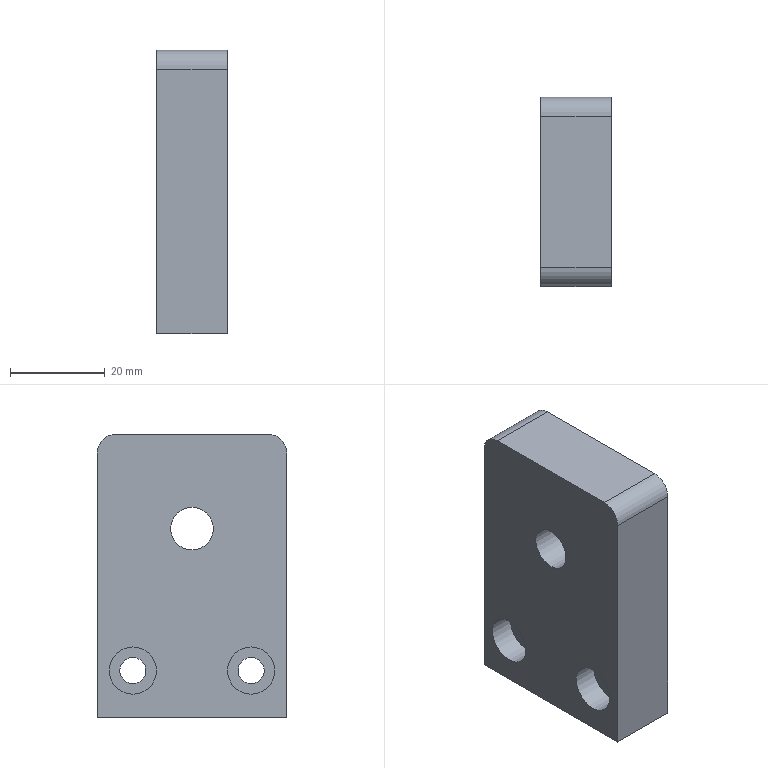Part | NX | 1 solid | 17 faces | box 15 x 40 x 60 mm | volume 32666 mm3 | plane 9 | cylinder 8 | commonest cylinder face diameters 5.5 x2 8 x2 10 x2 9 x1 15 x1
STEP:
#1=CARTESIAN_POINT('',(0.,-20.,-30.));
#2=VERTEX_POINT('',#1);
#3=CARTESIAN_POINT('',(0.,20.,-30.));
#4=VERTEX_POINT('',#3);
#5=CARTESIAN_POINT('',(0.,20.,-30.));
#6=DIRECTION('',(0.,1.,0.));
#7=VECTOR('',#6,1000.);
#8=LINE('',#5,#7);
#9=EDGE_CURVE('',#2,#4,#8,.T.);
#10=ORIENTED_EDGE('',*,*,#9,.T.);
#11=CARTESIAN_POINT('',(15.,20.,-30.));
#12=VERTEX_POINT('',#11);
#13=CARTESIAN_POINT('',(15.,20.,-30.));
#14=DIRECTION('',(-1.,0.,0.));
#15=VECTOR('',#14,1000.);
#16=LINE('',#13,#15);
#17=EDGE_CURVE('',#12,#4,#16,.T.);
#18=ORIENTED_EDGE('',*,*,#17,.F.);
#19=CARTESIAN_POINT('',(15.,-20.,-30.));
#20=VERTEX_POINT('',#19);
#21=CARTESIAN_POINT('',(15.,20.,-30.));
#22=DIRECTION('',(0.,1.,0.));
#23=VECTOR('',#22,1000.);
#24=LINE('',#21,#23);
#25=EDGE_CURVE('',#20,#12,#24,.T.);
#26=ORIENTED_EDGE('',*,*,#25,.F.);
#27=CARTESIAN_POINT('',(15.,-20.,-30.));
#28=DIRECTION('',(-1.,0.,0.));
#29=VECTOR('',#28,1000.);
#30=LINE('',#27,#29);
#31=EDGE_CURVE('',#20,#2,#30,.T.);
#32=ORIENTED_EDGE('',*,*,#31,.T.);
#33=EDGE_LOOP('',(#10,#18,#26,#32));
#34=FACE_BOUND('',#33,.T.);
#35=CARTESIAN_POINT('',(15.,20.,-30.));
#36=DIRECTION('',(0.,0.,1.));
#37=DIRECTION('',(1.,0.,0.));
#38=AXIS2_PLACEMENT_3D('',#35,#36,#37);
#39=PLANE('',#38);
#40=ADVANCED_FACE('',(#34),#39,.F.);
#41=CARTESIAN_POINT('',(0.,20.,26.));
#42=VERTEX_POINT('',#41);
#43=CARTESIAN_POINT('',(0.,20.,30.));
#44=DIRECTION('',(0.,0.,1.));
#45=VECTOR('',#44,1000.);
#46=LINE('',#43,#45);
#47=EDGE_CURVE('',#4,#42,#46,.T.);
#48=ORIENTED_EDGE('',*,*,#47,.T.);
#49=CARTESIAN_POINT('',(15.,20.,26.));
#50=VERTEX_POINT('',#49);
#51=CARTESIAN_POINT('',(15.,20.,26.));
#52=DIRECTION('',(-1.,0.,0.));
#53=VECTOR('',#52,1000.);
#54=LINE('',#51,#53);
#55=EDGE_CURVE('',#42,#50,#54,.F.);
#56=ORIENTED_EDGE('',*,*,#55,.T.);
#57=CARTESIAN_POINT('',(15.,20.,30.));
#58=DIRECTION('',(0.,0.,1.));
#59=VECTOR('',#58,1000.);
#60=LINE('',#57,#59);
#61=EDGE_CURVE('',#12,#50,#60,.T.);
#62=ORIENTED_EDGE('',*,*,#61,.F.);
#63=ORIENTED_EDGE('',*,*,#17,.T.);
#64=EDGE_LOOP('',(#48,#56,#62,#63));
#65=FACE_BOUND('',#64,.T.);
#66=CARTESIAN_POINT('',(15.,20.,30.));
#67=DIRECTION('',(0.,-1.,0.));
#68=DIRECTION('',(0.,0.,-1.));
#69=AXIS2_PLACEMENT_3D('',#66,#67,#68);
#70=PLANE('',#69);
#71=ADVANCED_FACE('',(#65),#70,.F.);
#72=CARTESIAN_POINT('',(0.,16.,30.));
#73=VERTEX_POINT('',#72);
#74=CARTESIAN_POINT('',(0.,-16.,30.));
#75=VERTEX_POINT('',#74);
#76=CARTESIAN_POINT('',(0.,20.,30.));
#77=DIRECTION('',(0.,-1.,0.));
#78=VECTOR('',#77,1000.);
#79=LINE('',#76,#78);
#80=EDGE_CURVE('',#73,#75,#79,.T.);
#81=ORIENTED_EDGE('',*,*,#80,.T.);
#82=CARTESIAN_POINT('',(15.,-16.,30.));
#83=VERTEX_POINT('',#82);
#84=CARTESIAN_POINT('',(15.,-16.,30.));
#85=DIRECTION('',(-1.,0.,0.));
#86=VECTOR('',#85,1000.);
#87=LINE('',#84,#86);
#88=EDGE_CURVE('',#75,#83,#87,.F.);
#89=ORIENTED_EDGE('',*,*,#88,.T.);
#90=CARTESIAN_POINT('',(15.,16.,30.));
#91=VERTEX_POINT('',#90);
#92=CARTESIAN_POINT('',(15.,20.,30.));
#93=DIRECTION('',(0.,-1.,0.));
#94=VECTOR('',#93,1000.);
#95=LINE('',#92,#94);
#96=EDGE_CURVE('',#91,#83,#95,.T.);
#97=ORIENTED_EDGE('',*,*,#96,.F.);
#98=CARTESIAN_POINT('',(15.,16.,30.));
#99=DIRECTION('',(-1.,0.,0.));
#100=VECTOR('',#99,1000.);
#101=LINE('',#98,#100);
#102=EDGE_CURVE('',#91,#73,#101,.T.);
#103=ORIENTED_EDGE('',*,*,#102,.T.);
#104=EDGE_LOOP('',(#81,#89,#97,#103));
#105=FACE_BOUND('',#104,.T.);
#106=CARTESIAN_POINT('',(15.,20.,30.));
#107=DIRECTION('',(0.,0.,-1.));
#108=DIRECTION('',(0.,1.,0.));
#109=AXIS2_PLACEMENT_3D('',#106,#107,#108);
#110=PLANE('',#109);
#111=ADVANCED_FACE('',(#105),#110,.F.);
#112=CARTESIAN_POINT('',(15.,-20.,26.));
#113=VERTEX_POINT('',#112);
#114=CARTESIAN_POINT('',(15.,-20.,30.));
#115=DIRECTION('',(0.,0.,-1.));
#116=VECTOR('',#115,1000.);
#117=LINE('',#114,#116);
#118=EDGE_CURVE('',#113,#20,#117,.T.);
#119=ORIENTED_EDGE('',*,*,#118,.F.);
#120=CARTESIAN_POINT('',(0.,-20.,26.));
#121=VERTEX_POINT('',#120);
#122=CARTESIAN_POINT('',(15.,-20.,26.));
#123=DIRECTION('',(-1.,0.,0.));
#124=VECTOR('',#123,1000.);
#125=LINE('',#122,#124);
#126=EDGE_CURVE('',#113,#121,#125,.T.);
#127=ORIENTED_EDGE('',*,*,#126,.T.);
#128=CARTESIAN_POINT('',(0.,-20.,30.));
#129=DIRECTION('',(0.,0.,-1.));
#130=VECTOR('',#129,1000.);
#131=LINE('',#128,#130);
#132=EDGE_CURVE('',#121,#2,#131,.T.);
#133=ORIENTED_EDGE('',*,*,#132,.T.);
#134=ORIENTED_EDGE('',*,*,#31,.F.);
#135=EDGE_LOOP('',(#119,#127,#133,#134));
#136=FACE_BOUND('',#135,.T.);
#137=CARTESIAN_POINT('',(15.,-20.,30.));
#138=DIRECTION('',(0.,1.,0.));
#139=DIRECTION('',(0.,0.,1.));
#140=AXIS2_PLACEMENT_3D('',#137,#138,#139);
#141=PLANE('',#140);
#142=ADVANCED_FACE('',(#136),#141,.F.);
#143=CARTESIAN_POINT('',(15.,-12.5,-17.25));
#144=VERTEX_POINT('',#143);
#145=CARTESIAN_POINT('',(15.,-12.5,-20.));
#146=DIRECTION('',(-1.,0.,0.));
#147=DIRECTION('',(0.,0.,1.));
#148=AXIS2_PLACEMENT_3D('',#145,#146,#147);
#149=CIRCLE('',#148,2.75);
#150=EDGE_CURVE('',#144,#144,#149,.T.);
#151=ORIENTED_EDGE('',*,*,#150,.T.);
#152=EDGE_LOOP('',(#151));
#153=FACE_BOUND('',#152,.T.);
#154=CARTESIAN_POINT('',(15.,12.5,-17.25));
#155=VERTEX_POINT('',#154);
#156=CARTESIAN_POINT('',(15.,12.5,-20.));
#157=DIRECTION('',(-1.,0.,0.));
#158=DIRECTION('',(0.,0.,1.));
#159=AXIS2_PLACEMENT_3D('',#156,#157,#158);
#160=CIRCLE('',#159,2.75);
#161=EDGE_CURVE('',#155,#155,#160,.T.);
#162=ORIENTED_EDGE('',*,*,#161,.T.);
#163=EDGE_LOOP('',(#162));
#164=FACE_BOUND('',#163,.T.);
#165=CARTESIAN_POINT('',(15.,0.,2.5));
#166=VERTEX_POINT('',#165);
#167=CARTESIAN_POINT('',(15.,0.,10.));
#168=DIRECTION('',(1.,0.,0.));
#169=DIRECTION('',(0.,0.,-1.));
#170=AXIS2_PLACEMENT_3D('',#167,#168,#169);
#171=CIRCLE('',#170,7.5);
#172=EDGE_CURVE('',#166,#166,#171,.T.);
#173=ORIENTED_EDGE('',*,*,#172,.F.);
#174=EDGE_LOOP('',(#173));
#175=FACE_BOUND('',#174,.T.);
#176=ORIENTED_EDGE('',*,*,#96,.T.);
#177=CARTESIAN_POINT('',(15.,-16.,26.));
#178=DIRECTION('',(1.,0.,0.));
#179=DIRECTION('',(0.,0.,-1.));
#180=AXIS2_PLACEMENT_3D('',#177,#178,#179);
#181=CIRCLE('',#180,4.);
#182=EDGE_CURVE('',#83,#113,#181,.T.);
#183=ORIENTED_EDGE('',*,*,#182,.T.);
#184=ORIENTED_EDGE('',*,*,#118,.T.);
#185=ORIENTED_EDGE('',*,*,#25,.T.);
#186=ORIENTED_EDGE('',*,*,#61,.T.);
#187=CARTESIAN_POINT('',(15.,16.,26.));
#188=DIRECTION('',(1.,0.,0.));
#189=DIRECTION('',(0.,0.,-1.));
#190=AXIS2_PLACEMENT_3D('',#187,#188,#189);
#191=CIRCLE('',#190,4.);
#192=EDGE_CURVE('',#50,#91,#191,.T.);
#193=ORIENTED_EDGE('',*,*,#192,.T.);
#194=EDGE_LOOP('',(#176,#183,#184,#185,#186,#193));
#195=FACE_BOUND('',#194,.T.);
#196=CARTESIAN_POINT('',(15.,0.,0.));
#197=DIRECTION('',(1.,0.,0.));
#198=DIRECTION('',(0.,0.,-1.));
#199=AXIS2_PLACEMENT_3D('',#196,#197,#198);
#200=PLANE('',#199);
#201=ADVANCED_FACE('',(#153,#164,#175,#195),#200,.T.);
#202=CARTESIAN_POINT('',(0.,-12.5,-15.));
#203=VERTEX_POINT('',#202);
#204=CARTESIAN_POINT('',(0.,-12.5,-20.));
#205=DIRECTION('',(-1.,0.,0.));
#206=DIRECTION('',(0.,0.,1.));
#207=AXIS2_PLACEMENT_3D('',#204,#205,#206);
#208=CIRCLE('',#207,5.);
#209=EDGE_CURVE('',#203,#203,#208,.T.);
#210=ORIENTED_EDGE('',*,*,#209,.F.);
#211=EDGE_LOOP('',(#210));
#212=FACE_BOUND('',#211,.T.);
#213=CARTESIAN_POINT('',(0.,12.5,-15.));
#214=VERTEX_POINT('',#213);
#215=CARTESIAN_POINT('',(0.,12.5,-20.));
#216=DIRECTION('',(-1.,0.,0.));
#217=DIRECTION('',(0.,0.,1.));
#218=AXIS2_PLACEMENT_3D('',#215,#216,#217);
#219=CIRCLE('',#218,5.);
#220=EDGE_CURVE('',#214,#214,#219,.T.);
#221=ORIENTED_EDGE('',*,*,#220,.F.);
#222=EDGE_LOOP('',(#221));
#223=FACE_BOUND('',#222,.T.);
#224=CARTESIAN_POINT('',(0.,0.,5.5));
#225=VERTEX_POINT('',#224);
#226=CARTESIAN_POINT('',(0.,0.,10.));
#227=DIRECTION('',(1.,0.,0.));
#228=DIRECTION('',(0.,0.,-1.));
#229=AXIS2_PLACEMENT_3D('',#226,#227,#228);
#230=CIRCLE('',#229,4.5);
#231=EDGE_CURVE('',#225,#225,#230,.T.);
#232=ORIENTED_EDGE('',*,*,#231,.T.);
#233=EDGE_LOOP('',(#232));
#234=FACE_BOUND('',#233,.T.);
#235=ORIENTED_EDGE('',*,*,#132,.F.);
#236=CARTESIAN_POINT('',(0.,-16.,26.));
#237=DIRECTION('',(1.,0.,0.));
#238=DIRECTION('',(0.,0.,-1.));
#239=AXIS2_PLACEMENT_3D('',#236,#237,#238);
#240=CIRCLE('',#239,4.);
#241=EDGE_CURVE('',#121,#75,#240,.F.);
#242=ORIENTED_EDGE('',*,*,#241,.T.);
#243=ORIENTED_EDGE('',*,*,#80,.F.);
#244=CARTESIAN_POINT('',(0.,16.,26.));
#245=DIRECTION('',(1.,0.,0.));
#246=DIRECTION('',(0.,0.,-1.));
#247=AXIS2_PLACEMENT_3D('',#244,#245,#246);
#248=CIRCLE('',#247,4.);
#249=EDGE_CURVE('',#73,#42,#248,.F.);
#250=ORIENTED_EDGE('',*,*,#249,.T.);
#251=ORIENTED_EDGE('',*,*,#47,.F.);
#252=ORIENTED_EDGE('',*,*,#9,.F.);
#253=EDGE_LOOP('',(#235,#242,#243,#250,#251,#252));
#254=FACE_BOUND('',#253,.T.);
#255=CARTESIAN_POINT('',(0.,0.,0.));
#256=DIRECTION('',(1.,0.,0.));
#257=DIRECTION('',(0.,0.,-1.));
#258=AXIS2_PLACEMENT_3D('',#255,#256,#257);
#259=PLANE('',#258);
#260=ADVANCED_FACE('',(#212,#223,#234,#254),#259,.F.);
#261=ORIENTED_EDGE('',*,*,#231,.F.);
#262=EDGE_LOOP('',(#261));
#263=FACE_BOUND('',#262,.T.);
#264=CARTESIAN_POINT('',(6.4,0.,5.5));
#265=VERTEX_POINT('',#264);
#266=CARTESIAN_POINT('',(6.4,0.,10.));
#267=DIRECTION('',(1.,0.,0.));
#268=DIRECTION('',(0.,0.,-1.));
#269=AXIS2_PLACEMENT_3D('',#266,#267,#268);
#270=CIRCLE('',#269,4.5);
#271=EDGE_CURVE('',#265,#265,#270,.T.);
#272=ORIENTED_EDGE('',*,*,#271,.T.);
#273=EDGE_LOOP('',(#272));
#274=FACE_BOUND('',#273,.T.);
#275=CARTESIAN_POINT('',(15.,0.,10.));
#276=DIRECTION('',(1.,0.,0.));
#277=DIRECTION('',(0.,0.,-1.));
#278=AXIS2_PLACEMENT_3D('',#275,#276,#277);
#279=CYLINDRICAL_SURFACE('',#278,4.5);
#280=ADVANCED_FACE('',(#263,#274),#279,.F.);
#281=ORIENTED_EDGE('',*,*,#271,.F.);
#282=EDGE_LOOP('',(#281));
#283=FACE_BOUND('',#282,.T.);
#284=CARTESIAN_POINT('',(6.4,0.,2.5));
#285=VERTEX_POINT('',#284);
#286=CARTESIAN_POINT('',(6.4,0.,10.));
#287=DIRECTION('',(1.,0.,0.));
#288=DIRECTION('',(0.,0.,-1.));
#289=AXIS2_PLACEMENT_3D('',#286,#287,#288);
#290=CIRCLE('',#289,7.5);
#291=EDGE_CURVE('',#285,#285,#290,.T.);
#292=ORIENTED_EDGE('',*,*,#291,.T.);
#293=EDGE_LOOP('',(#292));
#294=FACE_BOUND('',#293,.T.);
#295=CARTESIAN_POINT('',(6.4,4.5,10.));
#296=DIRECTION('',(-1.,0.,0.));
#297=DIRECTION('',(0.,0.,1.));
#298=AXIS2_PLACEMENT_3D('',#295,#296,#297);
#299=PLANE('',#298);
#300=ADVANCED_FACE('',(#283,#294),#299,.F.);
#301=ORIENTED_EDGE('',*,*,#291,.F.);
#302=EDGE_LOOP('',(#301));
#303=FACE_BOUND('',#302,.T.);
#304=ORIENTED_EDGE('',*,*,#172,.T.);
#305=EDGE_LOOP('',(#304));
#306=FACE_BOUND('',#305,.T.);
#307=CARTESIAN_POINT('',(15.,0.,10.));
#308=DIRECTION('',(1.,0.,0.));
#309=DIRECTION('',(0.,0.,-1.));
#310=AXIS2_PLACEMENT_3D('',#307,#308,#309);
#311=CYLINDRICAL_SURFACE('',#310,7.5);
#312=ADVANCED_FACE('',(#303,#306),#311,.F.);
#313=ORIENTED_EDGE('',*,*,#161,.F.);
#314=EDGE_LOOP('',(#313));
#315=FACE_BOUND('',#314,.T.);
#316=CARTESIAN_POINT('',(5.4,12.5,-17.25));
#317=VERTEX_POINT('',#316);
#318=CARTESIAN_POINT('',(5.4,12.5,-20.));
#319=DIRECTION('',(-1.,0.,0.));
#320=DIRECTION('',(0.,0.,1.));
#321=AXIS2_PLACEMENT_3D('',#318,#319,#320);
#322=CIRCLE('',#321,2.75);
#323=EDGE_CURVE('',#317,#317,#322,.T.);
#324=ORIENTED_EDGE('',*,*,#323,.T.);
#325=EDGE_LOOP('',(#324));
#326=FACE_BOUND('',#325,.T.);
#327=CARTESIAN_POINT('',(0.,12.5,-20.));
#328=DIRECTION('',(-1.,0.,0.));
#329=DIRECTION('',(0.,0.,1.));
#330=AXIS2_PLACEMENT_3D('',#327,#328,#329);
#331=CYLINDRICAL_SURFACE('',#330,2.75);
#332=ADVANCED_FACE('',(#315,#326),#331,.F.);
#333=ORIENTED_EDGE('',*,*,#323,.F.);
#334=EDGE_LOOP('',(#333));
#335=FACE_BOUND('',#334,.T.);
#336=CARTESIAN_POINT('',(5.4,12.5,-15.));
#337=VERTEX_POINT('',#336);
#338=CARTESIAN_POINT('',(5.4,12.5,-20.));
#339=DIRECTION('',(-1.,0.,0.));
#340=DIRECTION('',(0.,0.,1.));
#341=AXIS2_PLACEMENT_3D('',#338,#339,#340);
#342=CIRCLE('',#341,5.);
#343=EDGE_CURVE('',#337,#337,#342,.T.);
#344=ORIENTED_EDGE('',*,*,#343,.T.);
#345=EDGE_LOOP('',(#344));
#346=FACE_BOUND('',#345,.T.);
#347=CARTESIAN_POINT('',(5.4,15.25,-20.));
#348=DIRECTION('',(1.,0.,0.));
#349=DIRECTION('',(0.,0.,-1.));
#350=AXIS2_PLACEMENT_3D('',#347,#348,#349);
#351=PLANE('',#350);
#352=ADVANCED_FACE('',(#335,#346),#351,.F.);
#353=ORIENTED_EDGE('',*,*,#343,.F.);
#354=EDGE_LOOP('',(#353));
#355=FACE_BOUND('',#354,.T.);
#356=ORIENTED_EDGE('',*,*,#220,.T.);
#357=EDGE_LOOP('',(#356));
#358=FACE_BOUND('',#357,.T.);
#359=CARTESIAN_POINT('',(0.,12.5,-20.));
#360=DIRECTION('',(-1.,0.,0.));
#361=DIRECTION('',(0.,0.,1.));
#362=AXIS2_PLACEMENT_3D('',#359,#360,#361);
#363=CYLINDRICAL_SURFACE('',#362,5.);
#364=ADVANCED_FACE('',(#355,#358),#363,.F.);
#365=ORIENTED_EDGE('',*,*,#150,.F.);
#366=EDGE_LOOP('',(#365));
#367=FACE_BOUND('',#366,.T.);
#368=CARTESIAN_POINT('',(5.4,-12.5,-17.25));
#369=VERTEX_POINT('',#368);
#370=CARTESIAN_POINT('',(5.4,-12.5,-20.));
#371=DIRECTION('',(-1.,0.,0.));
#372=DIRECTION('',(0.,0.,1.));
#373=AXIS2_PLACEMENT_3D('',#370,#371,#372);
#374=CIRCLE('',#373,2.75);
#375=EDGE_CURVE('',#369,#369,#374,.T.);
#376=ORIENTED_EDGE('',*,*,#375,.T.);
#377=EDGE_LOOP('',(#376));
#378=FACE_BOUND('',#377,.T.);
#379=CARTESIAN_POINT('',(0.,-12.5,-20.));
#380=DIRECTION('',(-1.,0.,0.));
#381=DIRECTION('',(0.,0.,1.));
#382=AXIS2_PLACEMENT_3D('',#379,#380,#381);
#383=CYLINDRICAL_SURFACE('',#382,2.75);
#384=ADVANCED_FACE('',(#367,#378),#383,.F.);
#385=ORIENTED_EDGE('',*,*,#375,.F.);
#386=EDGE_LOOP('',(#385));
#387=FACE_BOUND('',#386,.T.);
#388=CARTESIAN_POINT('',(5.4,-12.5,-15.));
#389=VERTEX_POINT('',#388);
#390=CARTESIAN_POINT('',(5.4,-12.5,-20.));
#391=DIRECTION('',(-1.,0.,0.));
#392=DIRECTION('',(0.,0.,1.));
#393=AXIS2_PLACEMENT_3D('',#390,#391,#392);
#394=CIRCLE('',#393,5.);
#395=EDGE_CURVE('',#389,#389,#394,.T.);
#396=ORIENTED_EDGE('',*,*,#395,.T.);
#397=EDGE_LOOP('',(#396));
#398=FACE_BOUND('',#397,.T.);
#399=CARTESIAN_POINT('',(5.4,-9.75,-20.));
#400=DIRECTION('',(1.,0.,0.));
#401=DIRECTION('',(0.,0.,-1.));
#402=AXIS2_PLACEMENT_3D('',#399,#400,#401);
#403=PLANE('',#402);
#404=ADVANCED_FACE('',(#387,#398),#403,.F.);
#405=ORIENTED_EDGE('',*,*,#395,.F.);
#406=EDGE_LOOP('',(#405));
#407=FACE_BOUND('',#406,.T.);
#408=ORIENTED_EDGE('',*,*,#209,.T.);
#409=EDGE_LOOP('',(#408));
#410=FACE_BOUND('',#409,.T.);
#411=CARTESIAN_POINT('',(0.,-12.5,-20.));
#412=DIRECTION('',(-1.,0.,0.));
#413=DIRECTION('',(0.,0.,1.));
#414=AXIS2_PLACEMENT_3D('',#411,#412,#413);
#415=CYLINDRICAL_SURFACE('',#414,5.);
#416=ADVANCED_FACE('',(#407,#410),#415,.F.);
#417=ORIENTED_EDGE('',*,*,#182,.F.);
#418=ORIENTED_EDGE('',*,*,#88,.F.);
#419=ORIENTED_EDGE('',*,*,#241,.F.);
#420=ORIENTED_EDGE('',*,*,#126,.F.);
#421=EDGE_LOOP('',(#417,#418,#419,#420));
#422=FACE_BOUND('',#421,.T.);
#423=CARTESIAN_POINT('',(15.,-16.,26.));
#424=DIRECTION('',(-1.,0.,0.));
#425=DIRECTION('',(0.,0.,1.));
#426=AXIS2_PLACEMENT_3D('',#423,#424,#425);
#427=CYLINDRICAL_SURFACE('',#426,4.);
#428=ADVANCED_FACE('',(#422),#427,.T.);
#429=ORIENTED_EDGE('',*,*,#192,.F.);
#430=ORIENTED_EDGE('',*,*,#55,.F.);
#431=ORIENTED_EDGE('',*,*,#249,.F.);
#432=ORIENTED_EDGE('',*,*,#102,.F.);
#433=EDGE_LOOP('',(#429,#430,#431,#432));
#434=FACE_BOUND('',#433,.T.);
#435=CARTESIAN_POINT('',(15.,16.,26.));
#436=DIRECTION('',(-1.,0.,0.));
#437=DIRECTION('',(0.,0.,1.));
#438=AXIS2_PLACEMENT_3D('',#435,#436,#437);
#439=CYLINDRICAL_SURFACE('',#438,4.);
#440=ADVANCED_FACE('',(#434),#439,.T.);
#441=CLOSED_SHELL('',(#40,#71,#111,#142,#201,#260,#280,#300,#312,#332,#352,#364,#384,#404,#416,#428,#440));
#442=MANIFOLD_SOLID_BREP('',#441);
#443=(LENGTH_UNIT()NAMED_UNIT(*)SI_UNIT(.MILLI.,.METRE.));
#444=UNCERTAINTY_MEASURE_WITH_UNIT(LENGTH_MEASURE(0.00001),#443,'','');
#445=(NAMED_UNIT(*)PLANE_ANGLE_UNIT()SI_UNIT($,.RADIAN.));
#446=(NAMED_UNIT(*)SI_UNIT($,.STERADIAN.)SOLID_ANGLE_UNIT());
#447=(GEOMETRIC_REPRESENTATION_CONTEXT(3)GLOBAL_UNCERTAINTY_ASSIGNED_CONTEXT((#444))GLOBAL_UNIT_ASSIGNED_CONTEXT((#443,#445,#446))REPRESENTATION_CONTEXT('',''));
#448=ADVANCED_BREP_SHAPE_REPRESENTATION('',(#442),#447);